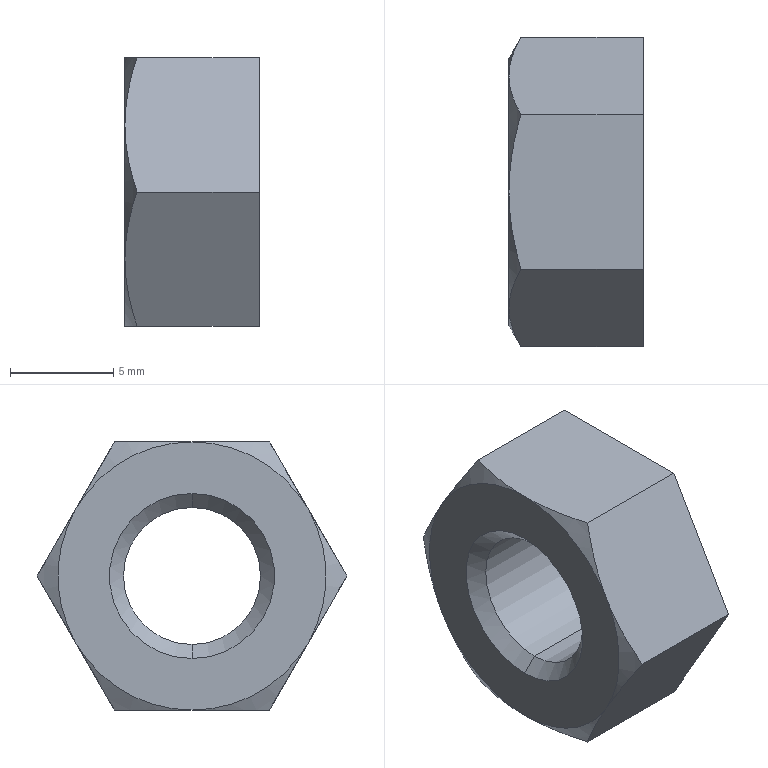Part | STEP file | 0228_312_SHNJ-M8 | 1 solid | 20 faces | box 6.5 x 15.011 x 13 mm | volume 713.151 mm3 | cone 10 | plane 8 | cylinder 2 | commonest cylinder face diameters 6.647 x2